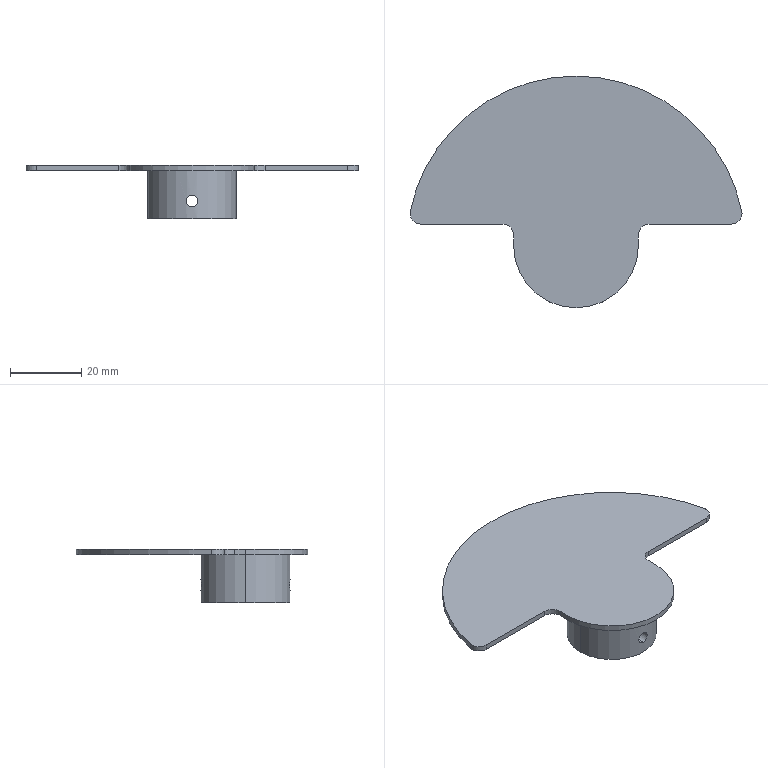Part | SolidWorks | features HoleWzd 3, Extrusion 1, Fillet 1, Revolution 1 | 1 solid | 23 faces | box 93.161 x 65 x 15 mm | volume 10485 mm3 | cylinder 15 | plane 8 | commonest cylinder face diameters 6 x5 3.3 x4 12 x2 25 x2 35 x1 95 x1
STEP:
#1=CARTESIAN_POINT('',(46.58,9.,-0.75));
#2=VERTEX_POINT('',#1);
#3=CARTESIAN_POINT('',(43.58,6.,-0.75));
#4=VERTEX_POINT('',#3);
#5=CARTESIAN_POINT('',(43.58,9.,-0.75));
#6=DIRECTION('',(0.,0.,-1.));
#7=DIRECTION('',(1.,0.,0.));
#8=AXIS2_PLACEMENT_3D('',#5,#6,#7);
#9=CIRCLE('',#8,3.);
#10=EDGE_CURVE('',#2,#4,#9,.T.);
#11=ORIENTED_EDGE('',*,*,#10,.F.);
#12=CARTESIAN_POINT('',(46.58,9.,0.75));
#13=VERTEX_POINT('',#12);
#14=CARTESIAN_POINT('',(46.58,9.,-0.75));
#15=DIRECTION('',(0.,0.,1.));
#16=VECTOR('',#15,1000.);
#17=LINE('',#14,#16);
#18=EDGE_CURVE('',#2,#13,#17,.T.);
#19=ORIENTED_EDGE('',*,*,#18,.T.);
#20=CARTESIAN_POINT('',(43.58,6.,0.75));
#21=VERTEX_POINT('',#20);
#22=CARTESIAN_POINT('',(43.58,9.,0.75));
#23=DIRECTION('',(0.,0.,1.));
#24=DIRECTION('',(1.,0.,0.));
#25=AXIS2_PLACEMENT_3D('',#22,#23,#24);
#26=CIRCLE('',#25,3.);
#27=EDGE_CURVE('',#21,#13,#26,.T.);
#28=ORIENTED_EDGE('',*,*,#27,.F.);
#29=CARTESIAN_POINT('',(43.58,6.,-0.75));
#30=DIRECTION('',(0.,0.,1.));
#31=VECTOR('',#30,1000.);
#32=LINE('',#29,#31);
#33=EDGE_CURVE('',#4,#21,#32,.T.);
#34=ORIENTED_EDGE('',*,*,#33,.F.);
#35=EDGE_LOOP('',(#11,#19,#28,#34));
#36=FACE_OUTER_BOUND('',#35,.T.);
#37=CARTESIAN_POINT('',(43.58,9.,-0.75));
#38=DIRECTION('',(0.,0.,1.));
#39=DIRECTION('',(1.,0.,0.));
#40=AXIS2_PLACEMENT_3D('',#37,#38,#39);
#41=CYLINDRICAL_SURFACE('',#40,3.);
#42=ADVANCED_FACE('',(#36),#41,.T.);
#43=CARTESIAN_POINT('',(0.,12.5,-10.9));
#44=VERTEX_POINT('',#43);
#45=CARTESIAN_POINT('',(0.,12.5,-7.6));
#46=VERTEX_POINT('',#45);
#47=CARTESIAN_POINT('',(0.,12.5,-10.9));
#48=CARTESIAN_POINT('',(-0.1091,12.5,-10.9));
#49=CARTESIAN_POINT('',(-0.2164,12.499,-10.889));
#50=CARTESIAN_POINT('',(-0.4275,12.493,-10.847));
#51=CARTESIAN_POINT('',(-0.5324,12.489,-10.815));
#52=CARTESIAN_POINT('',(-0.7322,12.479,-10.733));
#53=CARTESIAN_POINT('',(-0.8269,12.473,-10.682));
#54=CARTESIAN_POINT('',(-1.006,12.46,-10.562));
#55=CARTESIAN_POINT('',(-1.091,12.453,-10.493));
#56=CARTESIAN_POINT('',(-1.319,12.431,-10.264));
#57=CARTESIAN_POINT('',(-1.442,12.417,-10.08));
#58=CARTESIAN_POINT('',(-1.606,12.397,-9.683));
#59=CARTESIAN_POINT('',(-1.65,12.391,-9.466));
#60=CARTESIAN_POINT('',(-1.65,12.391,-9.143));
#61=CARTESIAN_POINT('',(-1.639,12.392,-9.033));
#62=CARTESIAN_POINT('',(-1.597,12.398,-8.822));
#63=CARTESIAN_POINT('',(-1.566,12.402,-8.719));
#64=CARTESIAN_POINT('',(-1.483,12.412,-8.519));
#65=CARTESIAN_POINT('',(-1.431,12.418,-8.422));
#66=CARTESIAN_POINT('',(-1.312,12.431,-8.244));
#67=CARTESIAN_POINT('',(-1.244,12.438,-8.16));
#68=CARTESIAN_POINT('',(-1.09,12.453,-8.006));
#69=CARTESIAN_POINT('',(-1.007,12.46,-7.938));
#70=CARTESIAN_POINT('',(-0.8281,12.473,-7.819));
#71=CARTESIAN_POINT('',(-0.7315,12.479,-7.767));
#72=CARTESIAN_POINT('',(-0.5318,12.489,-7.684));
#73=CARTESIAN_POINT('',(-0.4289,12.493,-7.653));
#74=CARTESIAN_POINT('',(-0.2172,12.499,-7.611));
#75=CARTESIAN_POINT('',(-0.1077,12.5,-7.6));
#76=CARTESIAN_POINT('',(0.,12.5,-7.6));
#77=B_SPLINE_CURVE_WITH_KNOTS('',3,(#47,#48,#49,#50,#51,#52,#53,#54,#55,#56,#57,#58,#59,#60,#61,#62,#63,#64,#65,#66,#67,#68,#69,#70,#71,#72,#73,#74,#75,#76),.UNSPECIFIED.,.F.,.F.,(4,2,2,2,2,2,2,2,2,2,2,2,2,2,4),(0.,0.0003228,0.0006455,0.0009683,0.001291,0.001937,0.002582,0.002905,0.003228,0.00355,0.003873,0.004196,0.004519,0.004842,0.005164),.UNSPECIFIED.);
#78=EDGE_CURVE('',#44,#46,#77,.T.);
#79=ORIENTED_EDGE('',*,*,#78,.T.);
#80=CARTESIAN_POINT('',(0.,6.,-7.6));
#81=VERTEX_POINT('',#80);
#82=CARTESIAN_POINT('',(0.,5.769,-7.6));
#83=DIRECTION('',(0.,-1.,0.));
#84=VECTOR('',#83,1000.);
#85=LINE('',#82,#84);
#86=EDGE_CURVE('',#46,#81,#85,.T.);
#87=ORIENTED_EDGE('',*,*,#86,.T.);
#88=CARTESIAN_POINT('',(0.,6.,-10.9));
#89=VERTEX_POINT('',#88);
#90=CARTESIAN_POINT('',(0.,6.,-10.9));
#91=CARTESIAN_POINT('',(-0.1096,6.,-10.9));
#92=CARTESIAN_POINT('',(-0.2172,5.997,-10.889));
#93=CARTESIAN_POINT('',(-0.4289,5.986,-10.847));
#94=CARTESIAN_POINT('',(-0.534,5.977,-10.815));
#95=CARTESIAN_POINT('',(-0.7336,5.956,-10.732));
#96=CARTESIAN_POINT('',(-0.8282,5.943,-10.681));
#97=CARTESIAN_POINT('',(-1.007,5.916,-10.561));
#98=CARTESIAN_POINT('',(-1.091,5.9,-10.492));
#99=CARTESIAN_POINT('',(-1.318,5.855,-10.265));
#100=CARTESIAN_POINT('',(-1.441,5.825,-10.082));
#101=CARTESIAN_POINT('',(-1.606,5.782,-9.685));
#102=CARTESIAN_POINT('',(-1.65,5.769,-9.467));
#103=CARTESIAN_POINT('',(-1.65,5.769,-9.143));
#104=CARTESIAN_POINT('',(-1.639,5.772,-9.033));
#105=CARTESIAN_POINT('',(-1.597,5.784,-8.821));
#106=CARTESIAN_POINT('',(-1.565,5.792,-8.717));
#107=CARTESIAN_POINT('',(-1.441,5.825,-8.417));
#108=CARTESIAN_POINT('',(-1.319,5.855,-8.235));
#109=CARTESIAN_POINT('',(-1.09,5.901,-8.007));
#110=CARTESIAN_POINT('',(-1.007,5.916,-7.939));
#111=CARTESIAN_POINT('',(-0.829,5.943,-7.819));
#112=CARTESIAN_POINT('',(-0.7323,5.956,-7.767));
#113=CARTESIAN_POINT('',(-0.5333,5.977,-7.685));
#114=CARTESIAN_POINT('',(-0.4304,5.985,-7.653));
#115=CARTESIAN_POINT('',(-0.2175,5.997,-7.611));
#116=CARTESIAN_POINT('',(-0.108,6.,-7.6));
#117=CARTESIAN_POINT('',(0.,6.,-7.6));
#118=B_SPLINE_CURVE_WITH_KNOTS('',3,(#90,#91,#92,#93,#94,#95,#96,#97,#98,#99,#100,#101,#102,#103,#104,#105,#106,#107,#108,#109,#110,#111,#112,#113,#114,#115,#116,#117),.UNSPECIFIED.,.F.,.F.,(4,2,2,2,2,2,2,2,2,2,2,2,2,4),(0.,0.000324,0.000648,0.000972,0.001296,0.001944,0.002592,0.002916,0.00324,0.003888,0.004212,0.004536,0.00486,0.005184),.UNSPECIFIED.);
#119=EDGE_CURVE('',#89,#81,#118,.T.);
#120=ORIENTED_EDGE('',*,*,#119,.F.);
#121=CARTESIAN_POINT('',(0.,5.769,-10.9));
#122=DIRECTION('',(0.,-1.,0.));
#123=VECTOR('',#122,1000.);
#124=LINE('',#121,#123);
#125=EDGE_CURVE('',#44,#89,#124,.T.);
#126=ORIENTED_EDGE('',*,*,#125,.F.);
#127=EDGE_LOOP('',(#79,#87,#120,#126));
#128=FACE_OUTER_BOUND('',#127,.T.);
#129=CARTESIAN_POINT('',(0.,5.769,-9.25));
#130=DIRECTION('',(0.,-1.,0.));
#131=DIRECTION('',(0.,0.,-1.));
#132=AXIS2_PLACEMENT_3D('',#129,#130,#131);
#133=CYLINDRICAL_SURFACE('',#132,1.65);
#134=ADVANCED_FACE('',(#128),#133,.F.);
#135=CARTESIAN_POINT('',(0.,-12.5,-7.6));
#136=VERTEX_POINT('',#135);
#137=CARTESIAN_POINT('',(0.,-12.5,-10.9));
#138=VERTEX_POINT('',#137);
#139=CARTESIAN_POINT('',(0.,-12.5,-7.6));
#140=CARTESIAN_POINT('',(-0.1091,-12.5,-7.6));
#141=CARTESIAN_POINT('',(-0.2164,-12.499,-7.611));
#142=CARTESIAN_POINT('',(-0.4275,-12.493,-7.653));
#143=CARTESIAN_POINT('',(-0.5324,-12.489,-7.685));
#144=CARTESIAN_POINT('',(-0.7322,-12.479,-7.767));
#145=CARTESIAN_POINT('',(-0.8269,-12.473,-7.818));
#146=CARTESIAN_POINT('',(-1.006,-12.46,-7.938));
#147=CARTESIAN_POINT('',(-1.091,-12.453,-8.007));
#148=CARTESIAN_POINT('',(-1.319,-12.431,-8.236));
#149=CARTESIAN_POINT('',(-1.442,-12.417,-8.42));
#150=CARTESIAN_POINT('',(-1.606,-12.397,-8.817));
#151=CARTESIAN_POINT('',(-1.65,-12.391,-9.034));
#152=CARTESIAN_POINT('',(-1.65,-12.391,-9.357));
#153=CARTESIAN_POINT('',(-1.639,-12.392,-9.467));
#154=CARTESIAN_POINT('',(-1.597,-12.398,-9.678));
#155=CARTESIAN_POINT('',(-1.566,-12.402,-9.781));
#156=CARTESIAN_POINT('',(-1.483,-12.412,-9.981));
#157=CARTESIAN_POINT('',(-1.431,-12.418,-10.078));
#158=CARTESIAN_POINT('',(-1.312,-12.431,-10.256));
#159=CARTESIAN_POINT('',(-1.244,-12.438,-10.34));
#160=CARTESIAN_POINT('',(-1.09,-12.453,-10.494));
#161=CARTESIAN_POINT('',(-1.007,-12.46,-10.562));
#162=CARTESIAN_POINT('',(-0.8281,-12.473,-10.681));
#163=CARTESIAN_POINT('',(-0.7315,-12.479,-10.733));
#164=CARTESIAN_POINT('',(-0.5318,-12.489,-10.816));
#165=CARTESIAN_POINT('',(-0.4289,-12.493,-10.847));
#166=CARTESIAN_POINT('',(-0.2172,-12.499,-10.889));
#167=CARTESIAN_POINT('',(-0.1077,-12.5,-10.9));
#168=CARTESIAN_POINT('',(0.,-12.5,-10.9));
#169=B_SPLINE_CURVE_WITH_KNOTS('',3,(#139,#140,#141,#142,#143,#144,#145,#146,#147,#148,#149,#150,#151,#152,#153,#154,#155,#156,#157,#158,#159,#160,#161,#162,#163,#164,#165,#166,#167,#168),.UNSPECIFIED.,.F.,.F.,(4,2,2,2,2,2,2,2,2,2,2,2,2,2,4),(0.,0.0003228,0.0006455,0.0009683,0.001291,0.001937,0.002582,0.002905,0.003228,0.00355,0.003873,0.004196,0.004519,0.004842,0.005164),.UNSPECIFIED.);
#170=EDGE_CURVE('',#136,#138,#169,.T.);
#171=ORIENTED_EDGE('',*,*,#170,.T.);
#172=CARTESIAN_POINT('',(0.,-6.,-10.9));
#173=VERTEX_POINT('',#172);
#174=CARTESIAN_POINT('',(0.,-5.769,-10.9));
#175=DIRECTION('',(0.,1.,0.));
#176=VECTOR('',#175,1000.);
#177=LINE('',#174,#176);
#178=EDGE_CURVE('',#138,#173,#177,.T.);
#179=ORIENTED_EDGE('',*,*,#178,.T.);
#180=CARTESIAN_POINT('',(0.,-6.,-7.6));
#181=VERTEX_POINT('',#180);
#182=CARTESIAN_POINT('',(0.,-6.,-7.6));
#183=CARTESIAN_POINT('',(-0.1096,-6.,-7.6));
#184=CARTESIAN_POINT('',(-0.2172,-5.997,-7.611));
#185=CARTESIAN_POINT('',(-0.4289,-5.986,-7.653));
#186=CARTESIAN_POINT('',(-0.534,-5.977,-7.685));
#187=CARTESIAN_POINT('',(-0.7336,-5.956,-7.768));
#188=CARTESIAN_POINT('',(-0.8282,-5.943,-7.819));
#189=CARTESIAN_POINT('',(-1.007,-5.916,-7.939));
#190=CARTESIAN_POINT('',(-1.091,-5.9,-8.008));
#191=CARTESIAN_POINT('',(-1.318,-5.855,-8.235));
#192=CARTESIAN_POINT('',(-1.441,-5.825,-8.418));
#193=CARTESIAN_POINT('',(-1.606,-5.782,-8.815));
#194=CARTESIAN_POINT('',(-1.65,-5.769,-9.033));
#195=CARTESIAN_POINT('',(-1.65,-5.769,-9.357));
#196=CARTESIAN_POINT('',(-1.639,-5.772,-9.467));
#197=CARTESIAN_POINT('',(-1.597,-5.784,-9.679));
#198=CARTESIAN_POINT('',(-1.565,-5.792,-9.783));
#199=CARTESIAN_POINT('',(-1.441,-5.825,-10.083));
#200=CARTESIAN_POINT('',(-1.319,-5.855,-10.265));
#201=CARTESIAN_POINT('',(-1.09,-5.901,-10.493));
#202=CARTESIAN_POINT('',(-1.007,-5.916,-10.561));
#203=CARTESIAN_POINT('',(-0.829,-5.943,-10.681));
#204=CARTESIAN_POINT('',(-0.7323,-5.956,-10.733));
#205=CARTESIAN_POINT('',(-0.5333,-5.977,-10.815));
#206=CARTESIAN_POINT('',(-0.4304,-5.985,-10.847));
#207=CARTESIAN_POINT('',(-0.2175,-5.997,-10.889));
#208=CARTESIAN_POINT('',(-0.108,-6.,-10.9));
#209=CARTESIAN_POINT('',(0.,-6.,-10.9));
#210=B_SPLINE_CURVE_WITH_KNOTS('',3,(#182,#183,#184,#185,#186,#187,#188,#189,#190,#191,#192,#193,#194,#195,#196,#197,#198,#199,#200,#201,#202,#203,#204,#205,#206,#207,#208,#209),.UNSPECIFIED.,.F.,.F.,(4,2,2,2,2,2,2,2,2,2,2,2,2,4),(0.,0.000324,0.000648,0.000972,0.001296,0.001944,0.002592,0.002916,0.00324,0.003888,0.004212,0.004536,0.00486,0.005184),.UNSPECIFIED.);
#211=EDGE_CURVE('',#181,#173,#210,.T.);
#212=ORIENTED_EDGE('',*,*,#211,.F.);
#213=CARTESIAN_POINT('',(0.,-5.769,-7.6));
#214=DIRECTION('',(0.,1.,0.));
#215=VECTOR('',#214,1000.);
#216=LINE('',#213,#215);
#217=EDGE_CURVE('',#136,#181,#216,.T.);
#218=ORIENTED_EDGE('',*,*,#217,.F.);
#219=EDGE_LOOP('',(#171,#179,#212,#218));
#220=FACE_OUTER_BOUND('',#219,.T.);
#221=CARTESIAN_POINT('',(0.,-5.769,-9.25));
#222=DIRECTION('',(0.,1.,0.));
#223=DIRECTION('',(0.,0.,1.));
#224=AXIS2_PLACEMENT_3D('',#221,#222,#223);
#225=CYLINDRICAL_SURFACE('',#224,1.65);
#226=ADVANCED_FACE('',(#220),#225,.F.);
#227=ORIENTED_EDGE('',*,*,#211,.T.);
#228=CARTESIAN_POINT('',(0.,-6.,-10.9));
#229=CARTESIAN_POINT('',(0.216,-6.,-10.9));
#230=CARTESIAN_POINT('',(0.434,-5.988,-10.856));
#231=CARTESIAN_POINT('',(0.7323,-5.956,-10.733));
#232=CARTESIAN_POINT('',(0.8288,-5.943,-10.681));
#233=CARTESIAN_POINT('',(1.008,-5.915,-10.561));
#234=CARTESIAN_POINT('',(1.09,-5.901,-10.493));
#235=CARTESIAN_POINT('',(1.243,-5.87,-10.341));
#236=CARTESIAN_POINT('',(1.312,-5.855,-10.257));
#237=CARTESIAN_POINT('',(1.431,-5.827,-10.079));
#238=CARTESIAN_POINT('',(1.482,-5.814,-9.984));
#239=CARTESIAN_POINT('',(1.565,-5.792,-9.783));
#240=CARTESIAN_POINT('',(1.597,-5.784,-9.68));
#241=CARTESIAN_POINT('',(1.639,-5.772,-9.468));
#242=CARTESIAN_POINT('',(1.65,-5.769,-9.359));
#243=CARTESIAN_POINT('',(1.65,-5.769,-9.142));
#244=CARTESIAN_POINT('',(1.639,-5.772,-9.034));
#245=CARTESIAN_POINT('',(1.597,-5.784,-8.822));
#246=CARTESIAN_POINT('',(1.565,-5.792,-8.717));
#247=CARTESIAN_POINT('',(1.441,-5.825,-8.418));
#248=CARTESIAN_POINT('',(1.319,-5.855,-8.235));
#249=CARTESIAN_POINT('',(1.016,-5.915,-7.932));
#250=CARTESIAN_POINT('',(0.8333,-5.945,-7.81));
#251=CARTESIAN_POINT('',(0.5352,-5.977,-7.685));
#252=CARTESIAN_POINT('',(0.4299,-5.986,-7.653));
#253=CARTESIAN_POINT('',(0.2174,-5.997,-7.611));
#254=CARTESIAN_POINT('',(0.1096,-6.,-7.6));
#255=CARTESIAN_POINT('',(0.,-6.,-7.6));
#256=B_SPLINE_CURVE_WITH_KNOTS('',3,(#228,#229,#230,#231,#232,#233,#234,#235,#236,#237,#238,#239,#240,#241,#242,#243,#244,#245,#246,#247,#248,#249,#250,#251,#252,#253,#254,#255),.UNSPECIFIED.,.F.,.F.,(4,2,2,2,2,2,2,2,2,2,2,2,2,4),(0.005184,0.005832,0.006155,0.006479,0.006803,0.007127,0.007451,0.007775,0.008099,0.008423,0.00907,0.009718,0.01004,0.01037),.UNSPECIFIED.);
#257=EDGE_CURVE('',#173,#181,#256,.T.);
#258=ORIENTED_EDGE('',*,*,#257,.T.);
#259=EDGE_LOOP('',(#227,#258));
#260=FACE_BOUND('',#259,.T.);
#261=CARTESIAN_POINT('',(6.,0.,-0.75));
#262=VERTEX_POINT('',#261);
#263=CARTESIAN_POINT('',(-6.,0.,-0.75));
#264=VERTEX_POINT('',#263);
#265=CARTESIAN_POINT('',(0.,0.,-0.75));
#266=DIRECTION('',(0.,0.,-1.));
#267=DIRECTION('',(-1.,0.,0.));
#268=AXIS2_PLACEMENT_3D('',#265,#266,#267);
#269=CIRCLE('',#268,6.);
#270=EDGE_CURVE('',#262,#264,#269,.T.);
#271=ORIENTED_EDGE('',*,*,#270,.F.);
#272=CARTESIAN_POINT('',(6.,0.,-14.25));
#273=VERTEX_POINT('',#272);
#274=CARTESIAN_POINT('',(6.,0.,-14.25));
#275=DIRECTION('',(0.,0.,-1.));
#276=VECTOR('',#275,1000.);
#277=LINE('',#274,#276);
#278=EDGE_CURVE('',#262,#273,#277,.T.);
#279=ORIENTED_EDGE('',*,*,#278,.T.);
#280=CARTESIAN_POINT('',(-6.,0.,-14.25));
#281=VERTEX_POINT('',#280);
#282=CARTESIAN_POINT('',(0.,0.,-14.25));
#283=DIRECTION('',(0.,0.,-1.));
#284=DIRECTION('',(-1.,0.,0.));
#285=AXIS2_PLACEMENT_3D('',#282,#283,#284);
#286=CIRCLE('',#285,6.);
#287=EDGE_CURVE('',#273,#281,#286,.T.);
#288=ORIENTED_EDGE('',*,*,#287,.T.);
#289=CARTESIAN_POINT('',(-6.,0.,-14.25));
#290=DIRECTION('',(0.,0.,-1.));
#291=VECTOR('',#290,1000.);
#292=LINE('',#289,#291);
#293=EDGE_CURVE('',#264,#281,#292,.T.);
#294=ORIENTED_EDGE('',*,*,#293,.F.);
#295=EDGE_LOOP('',(#271,#279,#288,#294));
#296=FACE_OUTER_BOUND('',#295,.T.);
#297=CARTESIAN_POINT('',(0.,0.,-14.25));
#298=DIRECTION('',(0.,0.,-1.));
#299=DIRECTION('',(-1.,0.,0.));
#300=AXIS2_PLACEMENT_3D('',#297,#298,#299);
#301=CYLINDRICAL_SURFACE('',#300,6.);
#302=ADVANCED_FACE('',(#260,#296),#301,.F.);
#303=ORIENTED_EDGE('',*,*,#78,.F.);
#304=CARTESIAN_POINT('',(0.,12.5,-7.6));
#305=CARTESIAN_POINT('',(0.2154,12.5,-7.6));
#306=CARTESIAN_POINT('',(0.4327,12.494,-7.643));
#307=CARTESIAN_POINT('',(0.8299,12.474,-7.808));
#308=CARTESIAN_POINT('',(1.014,12.46,-7.931));
#309=CARTESIAN_POINT('',(1.242,12.438,-8.158));
#310=CARTESIAN_POINT('',(1.312,12.431,-8.243));
#311=CARTESIAN_POINT('',(1.431,12.418,-8.422));
#312=CARTESIAN_POINT('',(1.482,12.412,-8.517));
#313=CARTESIAN_POINT('',(1.565,12.402,-8.717));
#314=CARTESIAN_POINT('',(1.597,12.398,-8.821));
#315=CARTESIAN_POINT('',(1.639,12.392,-9.032));
#316=CARTESIAN_POINT('',(1.65,12.391,-9.14));
#317=CARTESIAN_POINT('',(1.65,12.391,-9.358));
#318=CARTESIAN_POINT('',(1.639,12.392,-9.465));
#319=CARTESIAN_POINT('',(1.598,12.398,-9.676));
#320=CARTESIAN_POINT('',(1.566,12.402,-9.781));
#321=CARTESIAN_POINT('',(1.483,12.412,-9.981));
#322=CARTESIAN_POINT('',(1.433,12.418,-10.076));
#323=CARTESIAN_POINT('',(1.313,12.431,-10.255));
#324=CARTESIAN_POINT('',(1.243,12.438,-10.34));
#325=CARTESIAN_POINT('',(1.016,12.46,-10.568));
#326=CARTESIAN_POINT('',(0.8319,12.474,-10.691));
#327=CARTESIAN_POINT('',(0.4351,12.494,-10.856));
#328=CARTESIAN_POINT('',(0.2182,12.5,-10.9));
#329=CARTESIAN_POINT('',(0.,12.5,-10.9));
#330=B_SPLINE_CURVE_WITH_KNOTS('',3,(#304,#305,#306,#307,#308,#309,#310,#311,#312,#313,#314,#315,#316,#317,#318,#319,#320,#321,#322,#323,#324,#325,#326,#327,#328,#329),.UNSPECIFIED.,.F.,.F.,(4,2,2,2,2,2,2,2,2,2,2,2,4),(0.005164,0.00581,0.006455,0.006778,0.0071,0.007423,0.007746,0.008068,0.008391,0.008714,0.009037,0.009682,0.01033),.UNSPECIFIED.);
#331=EDGE_CURVE('',#46,#44,#330,.T.);
#332=ORIENTED_EDGE('',*,*,#331,.F.);
#333=EDGE_LOOP('',(#303,#332));
#334=FACE_BOUND('',#333,.T.);
#335=CARTESIAN_POINT('',(12.5,0.,-14.25));
#336=VERTEX_POINT('',#335);
#337=CARTESIAN_POINT('',(-12.5,0.,-14.25));
#338=VERTEX_POINT('',#337);
#339=CARTESIAN_POINT('',(0.,0.,-14.25));
#340=DIRECTION('',(0.,0.,1.));
#341=DIRECTION('',(1.,0.,0.));
#342=AXIS2_PLACEMENT_3D('',#339,#340,#341);
#343=CIRCLE('',#342,12.5);
#344=EDGE_CURVE('',#336,#338,#343,.T.);
#345=ORIENTED_EDGE('',*,*,#344,.T.);
#346=CARTESIAN_POINT('',(-12.5,0.,-0.75));
#347=VERTEX_POINT('',#346);
#348=CARTESIAN_POINT('',(-12.5,0.,-14.25));
#349=DIRECTION('',(0.,0.,1.));
#350=VECTOR('',#349,1000.);
#351=LINE('',#348,#350);
#352=EDGE_CURVE('',#338,#347,#351,.T.);
#353=ORIENTED_EDGE('',*,*,#352,.T.);
#354=CARTESIAN_POINT('',(12.5,0.,-0.75));
#355=VERTEX_POINT('',#354);
#356=CARTESIAN_POINT('',(0.,0.,-0.75));
#357=DIRECTION('',(0.,0.,1.));
#358=DIRECTION('',(1.,0.,0.));
#359=AXIS2_PLACEMENT_3D('',#356,#357,#358);
#360=CIRCLE('',#359,12.5);
#361=EDGE_CURVE('',#355,#347,#360,.T.);
#362=ORIENTED_EDGE('',*,*,#361,.F.);
#363=CARTESIAN_POINT('',(12.5,0.,-14.25));
#364=DIRECTION('',(0.,0.,1.));
#365=VECTOR('',#364,1000.);
#366=LINE('',#363,#365);
#367=EDGE_CURVE('',#336,#355,#366,.T.);
#368=ORIENTED_EDGE('',*,*,#367,.F.);
#369=EDGE_LOOP('',(#345,#353,#362,#368));
#370=FACE_OUTER_BOUND('',#369,.T.);
#371=CARTESIAN_POINT('',(0.,0.,-14.25));
#372=DIRECTION('',(0.,0.,1.));
#373=DIRECTION('',(1.,0.,0.));
#374=AXIS2_PLACEMENT_3D('',#371,#372,#373);
#375=CYLINDRICAL_SURFACE('',#374,12.5);
#376=ADVANCED_FACE('',(#334,#370),#375,.T.);
#377=CARTESIAN_POINT('',(17.5,0.,-0.75));
#378=VERTEX_POINT('',#377);
#379=CARTESIAN_POINT('',(17.5,3.,-0.75));
#380=VERTEX_POINT('',#379);
#381=CARTESIAN_POINT('',(17.5,0.,-0.75));
#382=DIRECTION('',(0.,1.,0.));
#383=VECTOR('',#382,1000.);
#384=LINE('',#381,#383);
#385=EDGE_CURVE('',#378,#380,#384,.T.);
#386=ORIENTED_EDGE('',*,*,#385,.T.);
#387=CARTESIAN_POINT('',(17.5,3.,0.75));
#388=VERTEX_POINT('',#387);
#389=CARTESIAN_POINT('',(17.5,3.,0.75));
#390=DIRECTION('',(0.,0.,1.));
#391=VECTOR('',#390,1000.);
#392=LINE('',#389,#391);
#393=EDGE_CURVE('',#380,#388,#392,.T.);
#394=ORIENTED_EDGE('',*,*,#393,.T.);
#395=CARTESIAN_POINT('',(17.5,0.,0.75));
#396=VERTEX_POINT('',#395);
#397=CARTESIAN_POINT('',(17.5,0.,0.75));
#398=DIRECTION('',(0.,1.,0.));
#399=VECTOR('',#398,1000.);
#400=LINE('',#397,#399);
#401=EDGE_CURVE('',#396,#388,#400,.T.);
#402=ORIENTED_EDGE('',*,*,#401,.F.);
#403=CARTESIAN_POINT('',(17.5,0.,-0.75));
#404=DIRECTION('',(0.,0.,1.));
#405=VECTOR('',#404,1000.);
#406=LINE('',#403,#405);
#407=EDGE_CURVE('',#378,#396,#406,.T.);
#408=ORIENTED_EDGE('',*,*,#407,.F.);
#409=EDGE_LOOP('',(#386,#394,#402,#408));
#410=FACE_OUTER_BOUND('',#409,.T.);
#411=CARTESIAN_POINT('',(17.5,0.,-0.75));
#412=DIRECTION('',(1.,0.,0.));
#413=DIRECTION('',(0.,1.,0.));
#414=AXIS2_PLACEMENT_3D('',#411,#412,#413);
#415=PLANE('',#414);
#416=ADVANCED_FACE('',(#410),#415,.T.);
#417=CARTESIAN_POINT('',(-17.5,0.,0.75));
#418=VERTEX_POINT('',#417);
#419=CARTESIAN_POINT('',(0.,0.,0.75));
#420=DIRECTION('',(0.,0.,1.));
#421=DIRECTION('',(1.,0.,0.));
#422=AXIS2_PLACEMENT_3D('',#419,#420,#421);
#423=CIRCLE('',#422,17.5);
#424=EDGE_CURVE('',#418,#396,#423,.T.);
#425=ORIENTED_EDGE('',*,*,#424,.F.);
#426=CARTESIAN_POINT('',(-17.5,0.,-0.75));
#427=VERTEX_POINT('',#426);
#428=CARTESIAN_POINT('',(-17.5,0.,-0.75));
#429=DIRECTION('',(0.,0.,1.));
#430=VECTOR('',#429,1000.);
#431=LINE('',#428,#430);
#432=EDGE_CURVE('',#427,#418,#431,.T.);
#433=ORIENTED_EDGE('',*,*,#432,.F.);
#434=CARTESIAN_POINT('',(0.,0.,-0.75));
#435=DIRECTION('',(0.,0.,1.));
#436=DIRECTION('',(1.,0.,0.));
#437=AXIS2_PLACEMENT_3D('',#434,#435,#436);
#438=CIRCLE('',#437,17.5);
#439=EDGE_CURVE('',#427,#378,#438,.T.);
#440=ORIENTED_EDGE('',*,*,#439,.T.);
#441=ORIENTED_EDGE('',*,*,#407,.T.);
#442=EDGE_LOOP('',(#425,#433,#440,#441));
#443=FACE_OUTER_BOUND('',#442,.T.);
#444=CARTESIAN_POINT('',(0.,0.,-0.75));
#445=DIRECTION('',(0.,0.,1.));
#446=DIRECTION('',(1.,0.,0.));
#447=AXIS2_PLACEMENT_3D('',#444,#445,#446);
#448=CYLINDRICAL_SURFACE('',#447,17.5);
#449=ADVANCED_FACE('',(#443),#448,.T.);
#450=CARTESIAN_POINT('',(-17.5,3.,0.75));
#451=VERTEX_POINT('',#450);
#452=CARTESIAN_POINT('',(-17.5,6.,0.75));
#453=DIRECTION('',(0.,-1.,0.));
#454=VECTOR('',#453,1000.);
#455=LINE('',#452,#454);
#456=EDGE_CURVE('',#451,#418,#455,.T.);
#457=ORIENTED_EDGE('',*,*,#456,.F.);
#458=CARTESIAN_POINT('',(-17.5,3.,-0.75));
#459=VERTEX_POINT('',#458);
#460=CARTESIAN_POINT('',(-17.5,3.,-0.75));
#461=DIRECTION('',(0.,0.,-1.));
#462=VECTOR('',#461,1000.);
#463=LINE('',#460,#462);
#464=EDGE_CURVE('',#451,#459,#463,.T.);
#465=ORIENTED_EDGE('',*,*,#464,.T.);
#466=CARTESIAN_POINT('',(-17.5,6.,-0.75));
#467=DIRECTION('',(0.,-1.,0.));
#468=VECTOR('',#467,1000.);
#469=LINE('',#466,#468);
#470=EDGE_CURVE('',#459,#427,#469,.T.);
#471=ORIENTED_EDGE('',*,*,#470,.T.);
#472=ORIENTED_EDGE('',*,*,#432,.T.);
#473=EDGE_LOOP('',(#457,#465,#471,#472));
#474=FACE_OUTER_BOUND('',#473,.T.);
#475=CARTESIAN_POINT('',(-17.5,6.,-0.75));
#476=DIRECTION('',(-1.,0.,0.));
#477=DIRECTION('',(0.,0.,1.));
#478=AXIS2_PLACEMENT_3D('',#475,#476,#477);
#479=PLANE('',#478);
#480=ADVANCED_FACE('',(#474),#479,.T.);
#481=CARTESIAN_POINT('',(-43.58,6.,-0.75));
#482=VERTEX_POINT('',#481);
#483=CARTESIAN_POINT('',(-20.5,6.,-0.75));
#484=VERTEX_POINT('',#483);
#485=CARTESIAN_POINT('',(-47.12,6.,-0.75));
#486=DIRECTION('',(1.,0.,0.));
#487=VECTOR('',#486,1000.);
#488=LINE('',#485,#487);
#489=EDGE_CURVE('',#482,#484,#488,.T.);
#490=ORIENTED_EDGE('',*,*,#489,.T.);
#491=CARTESIAN_POINT('',(-20.5,6.,0.75));
#492=VERTEX_POINT('',#491);
#493=CARTESIAN_POINT('',(-20.5,6.,0.75));
#494=DIRECTION('',(0.,0.,1.));
#495=VECTOR('',#494,1000.);
#496=LINE('',#493,#495);
#497=EDGE_CURVE('',#484,#492,#496,.T.);
#498=ORIENTED_EDGE('',*,*,#497,.T.);
#499=CARTESIAN_POINT('',(-43.58,6.,0.75));
#500=VERTEX_POINT('',#499);
#501=CARTESIAN_POINT('',(-47.12,6.,0.75));
#502=DIRECTION('',(1.,0.,0.));
#503=VECTOR('',#502,1000.);
#504=LINE('',#501,#503);
#505=EDGE_CURVE('',#500,#492,#504,.T.);
#506=ORIENTED_EDGE('',*,*,#505,.F.);
#507=CARTESIAN_POINT('',(-43.58,6.,-0.75));
#508=DIRECTION('',(0.,0.,-1.));
#509=VECTOR('',#508,1000.);
#510=LINE('',#507,#509);
#511=EDGE_CURVE('',#500,#482,#510,.T.);
#512=ORIENTED_EDGE('',*,*,#511,.T.);
#513=EDGE_LOOP('',(#490,#498,#506,#512));
#514=FACE_OUTER_BOUND('',#513,.T.);
#515=CARTESIAN_POINT('',(-47.12,6.,-0.75));
#516=DIRECTION('',(0.,-1.,0.));
#517=DIRECTION('',(1.,0.,0.));
#518=AXIS2_PLACEMENT_3D('',#515,#516,#517);
#519=PLANE('',#518);
#520=ADVANCED_FACE('',(#514),#519,.T.);
#521=CARTESIAN_POINT('',(46.518,9.607,-0.75));
#522=VERTEX_POINT('',#521);
#523=CARTESIAN_POINT('',(-46.518,9.607,-0.75));
#524=VERTEX_POINT('',#523);
#525=CARTESIAN_POINT('',(0.,0.,-0.75));
#526=DIRECTION('',(0.,0.,1.));
#527=DIRECTION('',(1.,0.,0.));
#528=AXIS2_PLACEMENT_3D('',#525,#526,#527);
#529=CIRCLE('',#528,47.5);
#530=EDGE_CURVE('',#522,#524,#529,.T.);
#531=ORIENTED_EDGE('',*,*,#530,.T.);
#532=CARTESIAN_POINT('',(-46.518,9.607,0.75));
#533=VERTEX_POINT('',#532);
#534=CARTESIAN_POINT('',(-46.518,9.607,-0.75));
#535=DIRECTION('',(0.,0.,1.));
#536=VECTOR('',#535,1000.);
#537=LINE('',#534,#536);
#538=EDGE_CURVE('',#524,#533,#537,.T.);
#539=ORIENTED_EDGE('',*,*,#538,.T.);
#540=CARTESIAN_POINT('',(46.518,9.607,0.75));
#541=VERTEX_POINT('',#540);
#542=CARTESIAN_POINT('',(0.,0.,0.75));
#543=DIRECTION('',(0.,0.,1.));
#544=DIRECTION('',(1.,0.,0.));
#545=AXIS2_PLACEMENT_3D('',#542,#543,#544);
#546=CIRCLE('',#545,47.5);
#547=EDGE_CURVE('',#541,#533,#546,.T.);
#548=ORIENTED_EDGE('',*,*,#547,.F.);
#549=CARTESIAN_POINT('',(46.518,9.607,-0.75));
#550=DIRECTION('',(0.,0.,-1.));
#551=VECTOR('',#550,1000.);
#552=LINE('',#549,#551);
#553=EDGE_CURVE('',#541,#522,#552,.T.);
#554=ORIENTED_EDGE('',*,*,#553,.T.);
#555=EDGE_LOOP('',(#531,#539,#548,#554));
#556=FACE_OUTER_BOUND('',#555,.T.);
#557=CARTESIAN_POINT('',(0.,0.,-0.75));
#558=DIRECTION('',(0.,0.,1.));
#559=DIRECTION('',(1.,0.,0.));
#560=AXIS2_PLACEMENT_3D('',#557,#558,#559);
#561=CYLINDRICAL_SURFACE('',#560,47.5);
#562=ADVANCED_FACE('',(#556),#561,.T.);
#563=CARTESIAN_POINT('',(20.5,6.,-0.75));
#564=VERTEX_POINT('',#563);
#565=CARTESIAN_POINT('',(17.5,6.,-0.75));
#566=DIRECTION('',(1.,0.,0.));
#567=VECTOR('',#566,1000.);
#568=LINE('',#565,#567);
#569=EDGE_CURVE('',#564,#4,#568,.T.);
#570=ORIENTED_EDGE('',*,*,#569,.T.);
#571=ORIENTED_EDGE('',*,*,#33,.T.);
#572=CARTESIAN_POINT('',(20.5,6.,0.75));
#573=VERTEX_POINT('',#572);
#574=CARTESIAN_POINT('',(17.5,6.,0.75));
#575=DIRECTION('',(1.,0.,0.));
#576=VECTOR('',#575,1000.);
#577=LINE('',#574,#576);
#578=EDGE_CURVE('',#573,#21,#577,.T.);
#579=ORIENTED_EDGE('',*,*,#578,.F.);
#580=CARTESIAN_POINT('',(20.5,6.,-0.75));
#581=DIRECTION('',(0.,0.,-1.));
#582=VECTOR('',#581,1000.);
#583=LINE('',#580,#582);
#584=EDGE_CURVE('',#573,#564,#583,.T.);
#585=ORIENTED_EDGE('',*,*,#584,.T.);
#586=EDGE_LOOP('',(#570,#571,#579,#585));
#587=FACE_OUTER_BOUND('',#586,.T.);
#588=CARTESIAN_POINT('',(17.5,6.,-0.75));
#589=DIRECTION('',(0.,-1.,0.));
#590=DIRECTION('',(1.,0.,0.));
#591=AXIS2_PLACEMENT_3D('',#588,#589,#590);
#592=PLANE('',#591);
#593=ADVANCED_FACE('',(#587),#592,.T.);
#594=ORIENTED_EDGE('',*,*,#361,.T.);
#595=CARTESIAN_POINT('',(0.,0.,-0.75));
#596=DIRECTION('',(0.,0.,1.));
#597=DIRECTION('',(1.,0.,0.));
#598=AXIS2_PLACEMENT_3D('',#595,#596,#597);
#599=CIRCLE('',#598,12.5);
#600=EDGE_CURVE('',#347,#355,#599,.T.);
#601=ORIENTED_EDGE('',*,*,#600,.T.);
#602=EDGE_LOOP('',(#594,#601));
#603=FACE_BOUND('',#602,.T.);
#604=ORIENTED_EDGE('',*,*,#489,.F.);
#605=CARTESIAN_POINT('',(-43.58,9.,-0.75));
#606=DIRECTION('',(0.,0.,-1.));
#607=DIRECTION('',(1.,0.,0.));
#608=AXIS2_PLACEMENT_3D('',#605,#606,#607);
#609=CIRCLE('',#608,3.);
#610=EDGE_CURVE('',#482,#524,#609,.T.);
#611=ORIENTED_EDGE('',*,*,#610,.T.);
#612=ORIENTED_EDGE('',*,*,#530,.F.);
#613=CARTESIAN_POINT('',(43.58,9.,-0.75));
#614=DIRECTION('',(0.,0.,-1.));
#615=DIRECTION('',(1.,0.,0.));
#616=AXIS2_PLACEMENT_3D('',#613,#614,#615);
#617=CIRCLE('',#616,3.);
#618=EDGE_CURVE('',#522,#2,#617,.T.);
#619=ORIENTED_EDGE('',*,*,#618,.T.);
#620=ORIENTED_EDGE('',*,*,#10,.T.);
#621=ORIENTED_EDGE('',*,*,#569,.F.);
#622=CARTESIAN_POINT('',(20.5,3.,-0.75));
#623=DIRECTION('',(0.,0.,1.));
#624=DIRECTION('',(1.,0.,0.));
#625=AXIS2_PLACEMENT_3D('',#622,#623,#624);
#626=CIRCLE('',#625,3.);
#627=EDGE_CURVE('',#564,#380,#626,.T.);
#628=ORIENTED_EDGE('',*,*,#627,.T.);
#629=ORIENTED_EDGE('',*,*,#385,.F.);
#630=ORIENTED_EDGE('',*,*,#439,.F.);
#631=ORIENTED_EDGE('',*,*,#470,.F.);
#632=CARTESIAN_POINT('',(-20.5,3.,-0.75));
#633=DIRECTION('',(0.,0.,1.));
#634=DIRECTION('',(1.,0.,0.));
#635=AXIS2_PLACEMENT_3D('',#632,#633,#634);
#636=CIRCLE('',#635,3.);
#637=EDGE_CURVE('',#459,#484,#636,.T.);
#638=ORIENTED_EDGE('',*,*,#637,.T.);
#639=EDGE_LOOP('',(#604,#611,#612,#619,#620,#621,#628,#629,#630,#631,#638));
#640=FACE_OUTER_BOUND('',#639,.T.);
#641=CARTESIAN_POINT('',(0.,0.,-0.75));
#642=DIRECTION('',(0.,0.,1.));
#643=DIRECTION('',(1.,0.,0.));
#644=AXIS2_PLACEMENT_3D('',#641,#642,#643);
#645=PLANE('',#644);
#646=ADVANCED_FACE('',(#603,#640),#645,.F.);
#647=ORIENTED_EDGE('',*,*,#547,.T.);
#648=CARTESIAN_POINT('',(-43.58,9.,0.75));
#649=DIRECTION('',(0.,0.,1.));
#650=DIRECTION('',(1.,0.,0.));
#651=AXIS2_PLACEMENT_3D('',#648,#649,#650);
#652=CIRCLE('',#651,3.);
#653=EDGE_CURVE('',#533,#500,#652,.T.);
#654=ORIENTED_EDGE('',*,*,#653,.T.);
#655=ORIENTED_EDGE('',*,*,#505,.T.);
#656=CARTESIAN_POINT('',(-20.5,3.,0.75));
#657=DIRECTION('',(0.,0.,-1.));
#658=DIRECTION('',(1.,0.,0.));
#659=AXIS2_PLACEMENT_3D('',#656,#657,#658);
#660=CIRCLE('',#659,3.);
#661=EDGE_CURVE('',#492,#451,#660,.T.);
#662=ORIENTED_EDGE('',*,*,#661,.T.);
#663=ORIENTED_EDGE('',*,*,#456,.T.);
#664=ORIENTED_EDGE('',*,*,#424,.T.);
#665=ORIENTED_EDGE('',*,*,#401,.T.);
#666=CARTESIAN_POINT('',(20.5,3.,0.75));
#667=DIRECTION('',(0.,0.,-1.));
#668=DIRECTION('',(1.,0.,0.));
#669=AXIS2_PLACEMENT_3D('',#666,#667,#668);
#670=CIRCLE('',#669,3.);
#671=EDGE_CURVE('',#388,#573,#670,.T.);
#672=ORIENTED_EDGE('',*,*,#671,.T.);
#673=ORIENTED_EDGE('',*,*,#578,.T.);
#674=ORIENTED_EDGE('',*,*,#27,.T.);
#675=CARTESIAN_POINT('',(43.58,9.,0.75));
#676=DIRECTION('',(0.,0.,1.));
#677=DIRECTION('',(1.,0.,0.));
#678=AXIS2_PLACEMENT_3D('',#675,#676,#677);
#679=CIRCLE('',#678,3.);
#680=EDGE_CURVE('',#13,#541,#679,.T.);
#681=ORIENTED_EDGE('',*,*,#680,.T.);
#682=EDGE_LOOP('',(#647,#654,#655,#662,#663,#664,#665,#672,#673,#674,#681));
#683=FACE_OUTER_BOUND('',#682,.T.);
#684=CARTESIAN_POINT('',(0.,0.,0.75));
#685=DIRECTION('',(0.,0.,1.));
#686=DIRECTION('',(1.,0.,0.));
#687=AXIS2_PLACEMENT_3D('',#684,#685,#686);
#688=PLANE('',#687);
#689=ADVANCED_FACE('',(#683),#688,.T.);
#690=ORIENTED_EDGE('',*,*,#352,.F.);
#691=CARTESIAN_POINT('',(0.,0.,-14.25));
#692=DIRECTION('',(0.,0.,1.));
#693=DIRECTION('',(1.,0.,0.));
#694=AXIS2_PLACEMENT_3D('',#691,#692,#693);
#695=CIRCLE('',#694,12.5);
#696=EDGE_CURVE('',#338,#336,#695,.T.);
#697=ORIENTED_EDGE('',*,*,#696,.T.);
#698=ORIENTED_EDGE('',*,*,#367,.T.);
#699=ORIENTED_EDGE('',*,*,#600,.F.);
#700=EDGE_LOOP('',(#690,#697,#698,#699));
#701=FACE_OUTER_BOUND('',#700,.T.);
#702=ORIENTED_EDGE('',*,*,#170,.F.);
#703=CARTESIAN_POINT('',(0.,-12.5,-10.9));
#704=CARTESIAN_POINT('',(0.2154,-12.5,-10.9));
#705=CARTESIAN_POINT('',(0.4327,-12.494,-10.857));
#706=CARTESIAN_POINT('',(0.8299,-12.474,-10.692));
#707=CARTESIAN_POINT('',(1.014,-12.46,-10.569));
#708=CARTESIAN_POINT('',(1.242,-12.438,-10.342));
#709=CARTESIAN_POINT('',(1.312,-12.431,-10.257));
#710=CARTESIAN_POINT('',(1.431,-12.418,-10.078));
#711=CARTESIAN_POINT('',(1.482,-12.412,-9.983));
#712=CARTESIAN_POINT('',(1.565,-12.402,-9.783));
#713=CARTESIAN_POINT('',(1.597,-12.398,-9.679));
#714=CARTESIAN_POINT('',(1.639,-12.392,-9.468));
#715=CARTESIAN_POINT('',(1.65,-12.391,-9.36));
#716=CARTESIAN_POINT('',(1.65,-12.391,-9.142));
#717=CARTESIAN_POINT('',(1.639,-12.392,-9.035));
#718=CARTESIAN_POINT('',(1.598,-12.398,-8.824));
#719=CARTESIAN_POINT('',(1.566,-12.402,-8.719));
#720=CARTESIAN_POINT('',(1.483,-12.412,-8.519));
#721=CARTESIAN_POINT('',(1.433,-12.418,-8.424));
#722=CARTESIAN_POINT('',(1.313,-12.431,-8.245));
#723=CARTESIAN_POINT('',(1.243,-12.438,-8.16));
#724=CARTESIAN_POINT('',(1.016,-12.46,-7.932));
#725=CARTESIAN_POINT('',(0.8319,-12.474,-7.809));
#726=CARTESIAN_POINT('',(0.4351,-12.494,-7.644));
#727=CARTESIAN_POINT('',(0.2182,-12.5,-7.6));
#728=CARTESIAN_POINT('',(0.,-12.5,-7.6));
#729=B_SPLINE_CURVE_WITH_KNOTS('',3,(#703,#704,#705,#706,#707,#708,#709,#710,#711,#712,#713,#714,#715,#716,#717,#718,#719,#720,#721,#722,#723,#724,#725,#726,#727,#728),.UNSPECIFIED.,.F.,.F.,(4,2,2,2,2,2,2,2,2,2,2,2,4),(0.005164,0.00581,0.006455,0.006778,0.0071,0.007423,0.007746,0.008068,0.008391,0.008714,0.009037,0.009682,0.01033),.UNSPECIFIED.);
#730=EDGE_CURVE('',#138,#136,#729,.T.);
#731=ORIENTED_EDGE('',*,*,#730,.F.);
#732=EDGE_LOOP('',(#702,#731));
#733=FACE_BOUND('',#732,.T.);
#734=CARTESIAN_POINT('',(0.,0.,-14.25));
#735=DIRECTION('',(0.,0.,1.));
#736=DIRECTION('',(1.,0.,0.));
#737=AXIS2_PLACEMENT_3D('',#734,#735,#736);
#738=CYLINDRICAL_SURFACE('',#737,12.5);
#739=ADVANCED_FACE('',(#701,#733),#738,.T.);
#740=CARTESIAN_POINT('',(0.,0.,-14.25));
#741=DIRECTION('',(0.,0.,-1.));
#742=DIRECTION('',(-1.,0.,0.));
#743=AXIS2_PLACEMENT_3D('',#740,#741,#742);
#744=CIRCLE('',#743,6.);
#745=EDGE_CURVE('',#281,#273,#744,.T.);
#746=ORIENTED_EDGE('',*,*,#745,.F.);
#747=ORIENTED_EDGE('',*,*,#287,.F.);
#748=EDGE_LOOP('',(#746,#747));
#749=FACE_BOUND('',#748,.T.);
#750=ORIENTED_EDGE('',*,*,#344,.F.);
#751=ORIENTED_EDGE('',*,*,#696,.F.);
#752=EDGE_LOOP('',(#750,#751));
#753=FACE_OUTER_BOUND('',#752,.T.);
#754=CARTESIAN_POINT('',(12.5,0.,-14.25));
#755=DIRECTION('',(0.,0.,-1.));
#756=DIRECTION('',(-1.,0.,0.));
#757=AXIS2_PLACEMENT_3D('',#754,#755,#756);
#758=PLANE('',#757);
#759=ADVANCED_FACE('',(#749,#753),#758,.T.);
#760=CARTESIAN_POINT('',(0.,0.,-0.75));
#761=DIRECTION('',(0.,0.,-1.));
#762=DIRECTION('',(-1.,0.,0.));
#763=AXIS2_PLACEMENT_3D('',#760,#761,#762);
#764=CIRCLE('',#763,6.);
#765=EDGE_CURVE('',#264,#262,#764,.T.);
#766=ORIENTED_EDGE('',*,*,#765,.T.);
#767=ORIENTED_EDGE('',*,*,#270,.T.);
#768=EDGE_LOOP('',(#766,#767));
#769=FACE_OUTER_BOUND('',#768,.T.);
#770=CARTESIAN_POINT('',(0.,0.,-0.75));
#771=DIRECTION('',(0.,0.,1.));
#772=DIRECTION('',(1.,0.,0.));
#773=AXIS2_PLACEMENT_3D('',#770,#771,#772);
#774=PLANE('',#773);
#775=ADVANCED_FACE('',(#769),#774,.F.);
#776=ORIENTED_EDGE('',*,*,#278,.F.);
#777=ORIENTED_EDGE('',*,*,#765,.F.);
#778=ORIENTED_EDGE('',*,*,#293,.T.);
#779=ORIENTED_EDGE('',*,*,#745,.T.);
#780=EDGE_LOOP('',(#776,#777,#778,#779));
#781=FACE_OUTER_BOUND('',#780,.T.);
#782=ORIENTED_EDGE('',*,*,#119,.T.);
#783=CARTESIAN_POINT('',(0.,6.,-7.6));
#784=CARTESIAN_POINT('',(0.216,6.,-7.6));
#785=CARTESIAN_POINT('',(0.434,5.988,-7.644));
#786=CARTESIAN_POINT('',(0.7323,5.956,-7.767));
#787=CARTESIAN_POINT('',(0.8288,5.943,-7.819));
#788=CARTESIAN_POINT('',(1.008,5.915,-7.939));
#789=CARTESIAN_POINT('',(1.09,5.901,-8.007));
#790=CARTESIAN_POINT('',(1.243,5.87,-8.159));
#791=CARTESIAN_POINT('',(1.312,5.855,-8.243));
#792=CARTESIAN_POINT('',(1.431,5.827,-8.421));
#793=CARTESIAN_POINT('',(1.482,5.814,-8.516));
#794=CARTESIAN_POINT('',(1.565,5.792,-8.717));
#795=CARTESIAN_POINT('',(1.597,5.784,-8.82));
#796=CARTESIAN_POINT('',(1.639,5.772,-9.032));
#797=CARTESIAN_POINT('',(1.65,5.769,-9.141));
#798=CARTESIAN_POINT('',(1.65,5.769,-9.358));
#799=CARTESIAN_POINT('',(1.639,5.772,-9.466));
#800=CARTESIAN_POINT('',(1.597,5.784,-9.678));
#801=CARTESIAN_POINT('',(1.565,5.792,-9.783));
#802=CARTESIAN_POINT('',(1.441,5.825,-10.082));
#803=CARTESIAN_POINT('',(1.319,5.855,-10.265));
#804=CARTESIAN_POINT('',(1.016,5.915,-10.568));
#805=CARTESIAN_POINT('',(0.8333,5.945,-10.69));
#806=CARTESIAN_POINT('',(0.5352,5.977,-10.815));
#807=CARTESIAN_POINT('',(0.4299,5.986,-10.847));
#808=CARTESIAN_POINT('',(0.2174,5.997,-10.889));
#809=CARTESIAN_POINT('',(0.1096,6.,-10.9));
#810=CARTESIAN_POINT('',(0.,6.,-10.9));
#811=B_SPLINE_CURVE_WITH_KNOTS('',3,(#783,#784,#785,#786,#787,#788,#789,#790,#791,#792,#793,#794,#795,#796,#797,#798,#799,#800,#801,#802,#803,#804,#805,#806,#807,#808,#809,#810),.UNSPECIFIED.,.F.,.F.,(4,2,2,2,2,2,2,2,2,2,2,2,2,4),(0.005184,0.005832,0.006155,0.006479,0.006803,0.007127,0.007451,0.007775,0.008099,0.008423,0.00907,0.009718,0.01004,0.01037),.UNSPECIFIED.);
#812=EDGE_CURVE('',#81,#89,#811,.T.);
#813=ORIENTED_EDGE('',*,*,#812,.T.);
#814=EDGE_LOOP('',(#782,#813));
#815=FACE_BOUND('',#814,.T.);
#816=CARTESIAN_POINT('',(0.,0.,-14.25));
#817=DIRECTION('',(0.,0.,-1.));
#818=DIRECTION('',(-1.,0.,0.));
#819=AXIS2_PLACEMENT_3D('',#816,#817,#818);
#820=CYLINDRICAL_SURFACE('',#819,6.);
#821=ADVANCED_FACE('',(#781,#815),#820,.F.);
#822=ORIENTED_EDGE('',*,*,#178,.F.);
#823=ORIENTED_EDGE('',*,*,#730,.T.);
#824=ORIENTED_EDGE('',*,*,#217,.T.);
#825=ORIENTED_EDGE('',*,*,#257,.F.);
#826=EDGE_LOOP('',(#822,#823,#824,#825));
#827=FACE_OUTER_BOUND('',#826,.T.);
#828=CARTESIAN_POINT('',(0.,-5.769,-9.25));
#829=DIRECTION('',(0.,1.,0.));
#830=DIRECTION('',(0.,0.,1.));
#831=AXIS2_PLACEMENT_3D('',#828,#829,#830);
#832=CYLINDRICAL_SURFACE('',#831,1.65);
#833=ADVANCED_FACE('',(#827),#832,.F.);
#834=ORIENTED_EDGE('',*,*,#86,.F.);
#835=ORIENTED_EDGE('',*,*,#331,.T.);
#836=ORIENTED_EDGE('',*,*,#125,.T.);
#837=ORIENTED_EDGE('',*,*,#812,.F.);
#838=EDGE_LOOP('',(#834,#835,#836,#837));
#839=FACE_OUTER_BOUND('',#838,.T.);
#840=CARTESIAN_POINT('',(0.,5.769,-9.25));
#841=DIRECTION('',(0.,-1.,0.));
#842=DIRECTION('',(0.,0.,-1.));
#843=AXIS2_PLACEMENT_3D('',#840,#841,#842);
#844=CYLINDRICAL_SURFACE('',#843,1.65);
#845=ADVANCED_FACE('',(#839),#844,.F.);
#846=ORIENTED_EDGE('',*,*,#637,.F.);
#847=ORIENTED_EDGE('',*,*,#464,.F.);
#848=ORIENTED_EDGE('',*,*,#661,.F.);
#849=ORIENTED_EDGE('',*,*,#497,.F.);
#850=EDGE_LOOP('',(#846,#847,#848,#849));
#851=FACE_OUTER_BOUND('',#850,.T.);
#852=CARTESIAN_POINT('',(-20.5,3.,-0.75));
#853=DIRECTION('',(0.,0.,-1.));
#854=DIRECTION('',(-1.,0.,0.));
#855=AXIS2_PLACEMENT_3D('',#852,#853,#854);
#856=CYLINDRICAL_SURFACE('',#855,3.);
#857=ADVANCED_FACE('',(#851),#856,.F.);
#858=ORIENTED_EDGE('',*,*,#610,.F.);
#859=ORIENTED_EDGE('',*,*,#511,.F.);
#860=ORIENTED_EDGE('',*,*,#653,.F.);
#861=ORIENTED_EDGE('',*,*,#538,.F.);
#862=EDGE_LOOP('',(#858,#859,#860,#861));
#863=FACE_OUTER_BOUND('',#862,.T.);
#864=CARTESIAN_POINT('',(-43.58,9.,-0.75));
#865=DIRECTION('',(0.,0.,1.));
#866=DIRECTION('',(1.,0.,0.));
#867=AXIS2_PLACEMENT_3D('',#864,#865,#866);
#868=CYLINDRICAL_SURFACE('',#867,3.);
#869=ADVANCED_FACE('',(#863),#868,.T.);
#870=ORIENTED_EDGE('',*,*,#18,.F.);
#871=ORIENTED_EDGE('',*,*,#618,.F.);
#872=ORIENTED_EDGE('',*,*,#553,.F.);
#873=ORIENTED_EDGE('',*,*,#680,.F.);
#874=EDGE_LOOP('',(#870,#871,#872,#873));
#875=FACE_OUTER_BOUND('',#874,.T.);
#876=CARTESIAN_POINT('',(43.58,9.,-0.75));
#877=DIRECTION('',(0.,0.,1.));
#878=DIRECTION('',(1.,0.,0.));
#879=AXIS2_PLACEMENT_3D('',#876,#877,#878);
#880=CYLINDRICAL_SURFACE('',#879,3.);
#881=ADVANCED_FACE('',(#875),#880,.T.);
#882=ORIENTED_EDGE('',*,*,#627,.F.);
#883=ORIENTED_EDGE('',*,*,#584,.F.);
#884=ORIENTED_EDGE('',*,*,#671,.F.);
#885=ORIENTED_EDGE('',*,*,#393,.F.);
#886=EDGE_LOOP('',(#882,#883,#884,#885));
#887=FACE_OUTER_BOUND('',#886,.T.);
#888=CARTESIAN_POINT('',(20.5,3.,-0.75));
#889=DIRECTION('',(0.,0.,-1.));
#890=DIRECTION('',(-1.,0.,0.));
#891=AXIS2_PLACEMENT_3D('',#888,#889,#890);
#892=CYLINDRICAL_SURFACE('',#891,3.);
#893=ADVANCED_FACE('',(#887),#892,.F.);
#894=CLOSED_SHELL('',(#42,#134,#226,#302,#376,#416,#449,#480,#520,#562,#593,#646,#689,#739,#759,#775,#821,#833,#845,#857,#869,#881,#893));
#895=MANIFOLD_SOLID_BREP('',#894);
#896=CARTESIAN_POINT('',(0.,0.,0.));
#897=DIRECTION('',(0.,0.,1.));
#898=DIRECTION('',(1.,0.,0.));
#899=AXIS2_PLACEMENT_3D('',#896,#897,#898);
#900=(LENGTH_UNIT()NAMED_UNIT(*)SI_UNIT(.MILLI.,.METRE.));
#901=UNCERTAINTY_MEASURE_WITH_UNIT(LENGTH_MEASURE(0.00001),#900,'','');
#902=(NAMED_UNIT(*)PLANE_ANGLE_UNIT()SI_UNIT($,.RADIAN.));
#903=(NAMED_UNIT(*)SI_UNIT($,.STERADIAN.)SOLID_ANGLE_UNIT());
#904=(GEOMETRIC_REPRESENTATION_CONTEXT(3)GLOBAL_UNCERTAINTY_ASSIGNED_CONTEXT((#901))GLOBAL_UNIT_ASSIGNED_CONTEXT((#900,#902,#903))REPRESENTATION_CONTEXT('',''));
#905=ADVANCED_BREP_SHAPE_REPRESENTATION('',(#895,#899),#904);